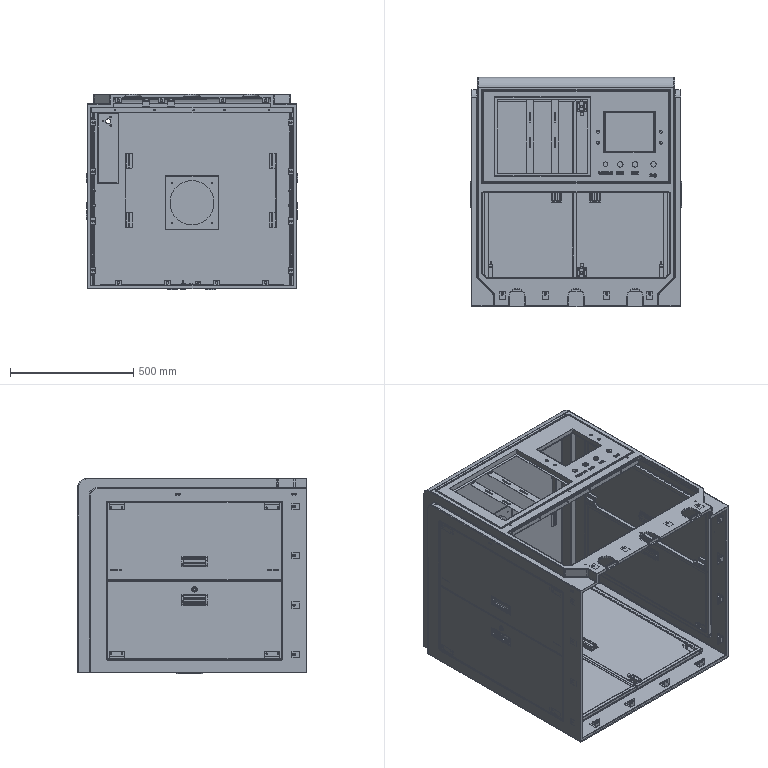Part | SolidWorks | features ReferencePattern 9, LocalLPattern 2 | 120 solids | 4016 faces | volume 7744813 mm3 | plane 2255 | cylinder 1455 | spline 161 | cone 74 | torus 67 | sphere 4 | commonest cylinder face diameters 6 x179 8 x136 1 x108 7 x89 4 x88 2.5 x72